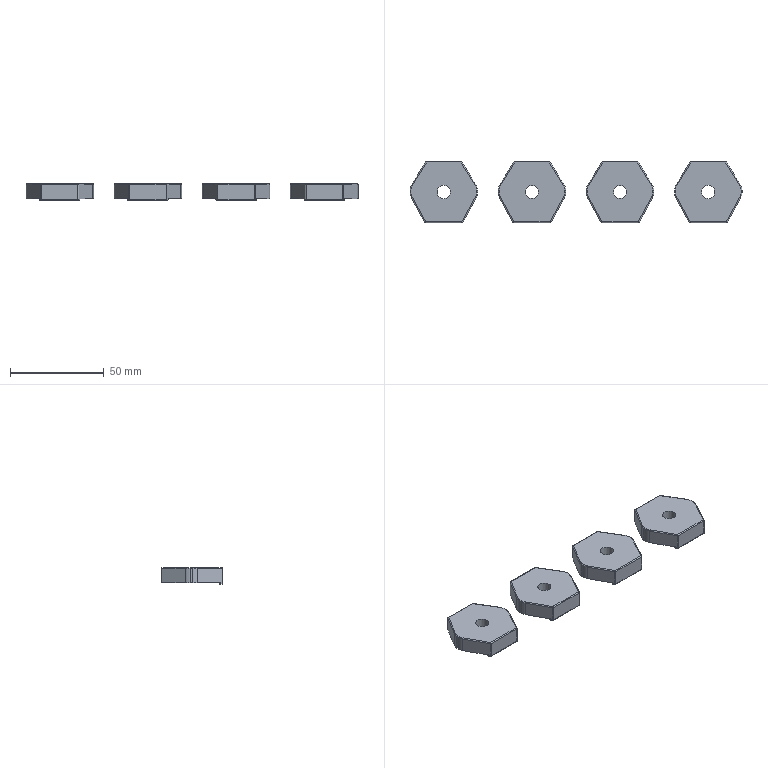CAM job | NX | 3-axis milling, drilling | part box 177 x 33 x 9 mm | stock box 182 x 35 x 12 mm
Tools:
number,name,description,diameter,corner_radius,flute_length,length,flutes
8,D8,平底铣刀-粗,8.0,0.0,30.0,75.0,2
9,D10,平底铣刀-粗,10.0,0.0,35.0,75.0,2
7,D6-J,平底铣刀-精,6.0,0.0,25.0,75.0,2
10,D10-J,平底铣刀-精,10.0,0.0,35.0,75.0,2
18,D6R0.5,圆鼻刀-粗,6.0,0.5,50.0,75.0,2
1,D80R0.8飞刀,圆鼻刀-粗,80.0,0.8,50.0,75.0,2
2,D6倒角刀,倒角刀,6.0,0.0,3.0,25.0,2
17,ZT7,钻头,7.0,0.0,35.0,50.0,2
Operations:
program,operation,operation_type,tool,method,geometry_group,spindle_rpm,surface_speed,feed_per_tooth,feed_cut,feed_plunge,cut_length_mm,path_length_mm,cut_time_min,machine_time_min
B,动态开粗D10_COPY_1,CavityMilling,D10,动态开粗-切深K-步距K,W-B,8000.0,251.32,0.25,4000.0,100.0,16350.389,16611.076,4.088,4.114
B,平面去毛刺6X45L_COPY,SurfaceContour,D6倒角刀,爬面_倒角-切深0-步距G,W-B,6500.0,122.519,0.1154,1500.0,100.0,473.586,879.389,0.3157,0.3563
B,等高螺旋爬面_COPY_COPY,ZLevelMilling,D6R0.5,等高爬面-切深K-步距G,W-B,7000.0,131.947,0.2857,4000.0,100.0,4365.673,4956.225,1.091,1.151
B,底壁铣精光底面-中_COPY,VolumeBased25DMillingOperation,D6-J,精光步距切深关,W-B,7000.0,175.0,0.0536,1500.0,100.0,158.13,245.662,0.1054,0.1142
B,底壁铣精光底面-中_COPY_1,VolumeBased25DMillingOperation,D6-J,精光步距切深关,W-B,7000.0,175.0,0.0536,1500.0,100.0,1388.195,1588.651,0.9255,0.9455
B,底壁铣精光侧面-中-选底面_COPY,VolumeBased25DMillingOperation,D6-J,侧刃精光-切深K-步距G,W-B,8000.0,150.792,0.0625,1000.0,100.0,162.994,263.172,0.163,0.173
A,顶面,FaceMilling,D80R0.8飞刀,侧刃精光-切深K-步距G,W-A,5000.0,1256.637,0.1,1000.0,100.0,271.0,307.0,0.271,0.2746
A,动态开粗D10_COPY,CavityMilling,D8,动态开粗-切深K-步距K,W-A,8000.0,201.062,0.2188,3500.0,100.0,7051.424,7106.024,2.015,2.02
A,打点-深0.8,Operation,D6倒角刀,NONE,W-A,8000.0,150.796,0.0312,500.0,90.0,7.2,198.432,0.0144,0.0335
A,通孔-6-8,Operation,ZT7,NONE,W-A,2500.0,54.978,0.06,300.0,90.0,52.412,288.856,0.1747,0.1984
A,等高螺旋爬面_COPY,ZLevelMilling,D6R0.5,等高爬面-切深K-步距G,W-A,7000.0,131.947,0.2857,4000.0,100.0,8979.562,9315.006,2.245,2.278
A,铣倒角_1,PlanarMilling,D6倒角刀,METHOD,W-A,8000.0,150.796,0.05,800.0,100.0,95.661,400.948,0.1196,0.1501
A,外形半精_2,VolumeBased25DMillingOperation,D10-J,METHOD,W-A,8000.0,251.327,0.0625,1000.0,100.0,598.497,957.015,0.5985,0.6343